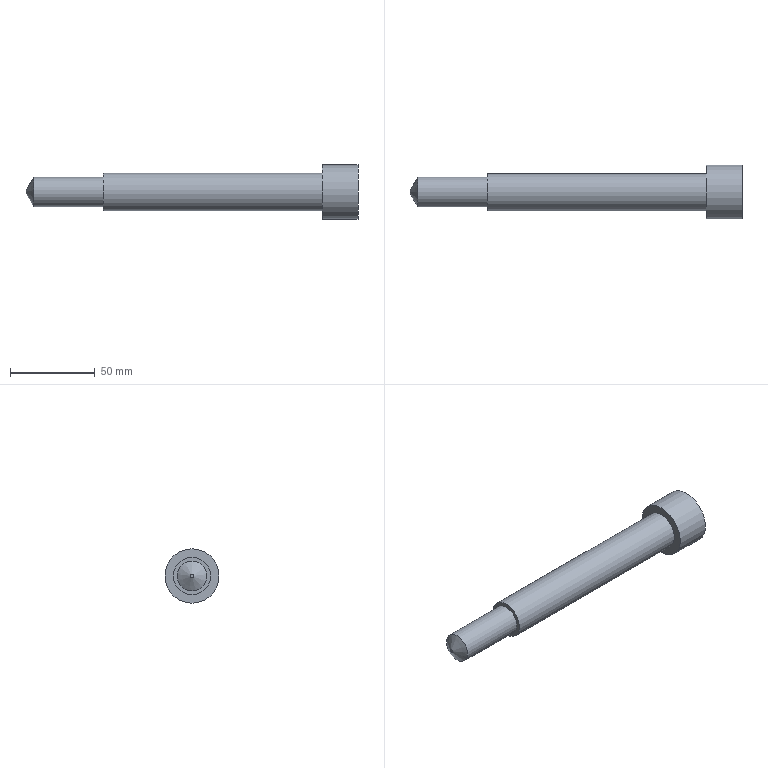Part | STEP file | solid 159 | 1 solid | 8 faces | box 195.5 x 32 x 32 mm | volume 76192 mm3 | plane 4 | cylinder 3 | cone 1 | commonest cylinder face diameters 17.5 x1 22 x1 32 x1